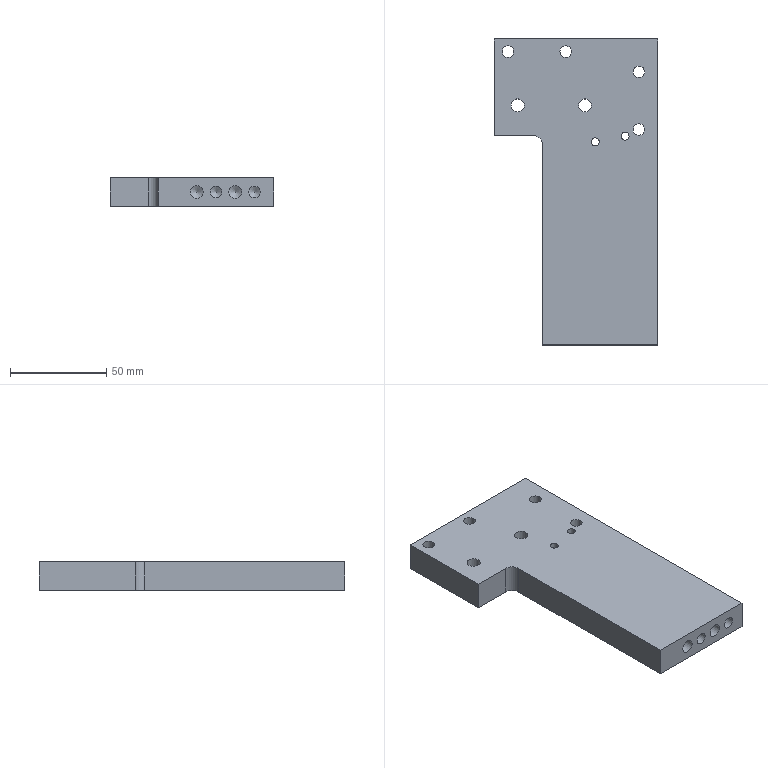Part | NX | features BREP 1 | 1 solid | 33 faces | box 85 x 159 x 15 mm | volume 154336 mm3 | cylinder 17 | plane 8 | cone 8 | commonest cylinder face diameters 6 x8 6.8 x6 4.2 x2 10 x1
STEP:
#1=CARTESIAN_POINT('',(-35.,-79.5,7.5));
#2=VERTEX_POINT('',#1);
#3=CARTESIAN_POINT('',(-35.,24.5,7.5));
#4=VERTEX_POINT('',#3);
#5=CARTESIAN_POINT('',(-35.,79.5,7.5));
#6=DIRECTION('',(0.,1.,0.));
#7=VECTOR('',#6,1000.);
#8=LINE('',#5,#7);
#9=EDGE_CURVE('',#2,#4,#8,.T.);
#10=ORIENTED_EDGE('',*,*,#9,.T.);
#11=CARTESIAN_POINT('',(-35.,24.5,-7.5));
#12=VERTEX_POINT('',#11);
#13=CARTESIAN_POINT('',(-35.,24.5,0.));
#14=DIRECTION('',(0.,0.,-1.));
#15=VECTOR('',#14,1000.);
#16=LINE('',#13,#15);
#17=EDGE_CURVE('',#4,#12,#16,.T.);
#18=ORIENTED_EDGE('',*,*,#17,.T.);
#19=CARTESIAN_POINT('',(-35.,-79.5,-7.5));
#20=VERTEX_POINT('',#19);
#21=CARTESIAN_POINT('',(-35.,79.5,-7.5));
#22=DIRECTION('',(0.,-1.,0.));
#23=VECTOR('',#22,1000.);
#24=LINE('',#21,#23);
#25=EDGE_CURVE('',#12,#20,#24,.T.);
#26=ORIENTED_EDGE('',*,*,#25,.T.);
#27=CARTESIAN_POINT('',(-35.,-79.5,7.5));
#28=DIRECTION('',(0.,0.,1.));
#29=VECTOR('',#28,1000.);
#30=LINE('',#27,#29);
#31=EDGE_CURVE('',#20,#2,#30,.T.);
#32=ORIENTED_EDGE('',*,*,#31,.T.);
#33=EDGE_LOOP('',(#10,#18,#26,#32));
#34=FACE_BOUND('',#33,.T.);
#35=CARTESIAN_POINT('',(-35.,0.,0.));
#36=DIRECTION('',(1.,0.,0.));
#37=DIRECTION('',(0.,0.,1.));
#38=AXIS2_PLACEMENT_3D('',#35,#36,#37);
#39=PLANE('',#38);
#40=ADVANCED_FACE('',(#34),#39,.F.);
#41=CARTESIAN_POINT('',(25.,-79.5,-7.5));
#42=VERTEX_POINT('',#41);
#43=CARTESIAN_POINT('',(25.,79.5,-7.5));
#44=VERTEX_POINT('',#43);
#45=CARTESIAN_POINT('',(25.,-79.5,-7.5));
#46=DIRECTION('',(0.,1.,0.));
#47=VECTOR('',#46,1000.);
#48=LINE('',#45,#47);
#49=EDGE_CURVE('',#42,#44,#48,.T.);
#50=ORIENTED_EDGE('',*,*,#49,.T.);
#51=CARTESIAN_POINT('',(25.,79.5,7.5));
#52=VERTEX_POINT('',#51);
#53=CARTESIAN_POINT('',(25.,79.5,7.5));
#54=DIRECTION('',(0.,0.,-1.));
#55=VECTOR('',#54,1000.);
#56=LINE('',#53,#55);
#57=EDGE_CURVE('',#52,#44,#56,.T.);
#58=ORIENTED_EDGE('',*,*,#57,.F.);
#59=CARTESIAN_POINT('',(25.,-79.5,7.5));
#60=VERTEX_POINT('',#59);
#61=CARTESIAN_POINT('',(25.,-79.5,7.5));
#62=DIRECTION('',(0.,1.,0.));
#63=VECTOR('',#62,1000.);
#64=LINE('',#61,#63);
#65=EDGE_CURVE('',#60,#52,#64,.T.);
#66=ORIENTED_EDGE('',*,*,#65,.F.);
#67=CARTESIAN_POINT('',(25.,-79.5,7.5));
#68=DIRECTION('',(0.,0.,-1.));
#69=VECTOR('',#68,1000.);
#70=LINE('',#67,#69);
#71=EDGE_CURVE('',#60,#42,#70,.T.);
#72=ORIENTED_EDGE('',*,*,#71,.T.);
#73=EDGE_LOOP('',(#50,#58,#66,#72));
#74=FACE_BOUND('',#73,.T.);
#75=CARTESIAN_POINT('',(25.,-79.5,7.5));
#76=DIRECTION('',(-1.,0.,0.));
#77=DIRECTION('',(0.,0.,-1.));
#78=AXIS2_PLACEMENT_3D('',#75,#76,#77);
#79=PLANE('',#78);
#80=ADVANCED_FACE('',(#74),#79,.F.);
#81=CARTESIAN_POINT('',(-5.,79.5,3.));
#82=VERTEX_POINT('',#81);
#83=CARTESIAN_POINT('',(-5.,79.5,0.));
#84=DIRECTION('',(0.,1.,0.));
#85=DIRECTION('',(0.,0.,1.));
#86=AXIS2_PLACEMENT_3D('',#83,#84,#85);
#87=CIRCLE('',#86,3.);
#88=EDGE_CURVE('',#82,#82,#87,.T.);
#89=ORIENTED_EDGE('',*,*,#88,.F.);
#90=EDGE_LOOP('',(#89));
#91=FACE_BOUND('',#90,.T.);
#92=CARTESIAN_POINT('',(15.,79.5,3.));
#93=VERTEX_POINT('',#92);
#94=CARTESIAN_POINT('',(15.,79.5,0.));
#95=DIRECTION('',(0.,1.,0.));
#96=DIRECTION('',(0.,0.,1.));
#97=AXIS2_PLACEMENT_3D('',#94,#95,#96);
#98=CIRCLE('',#97,3.);
#99=EDGE_CURVE('',#93,#93,#98,.T.);
#100=ORIENTED_EDGE('',*,*,#99,.F.);
#101=EDGE_LOOP('',(#100));
#102=FACE_BOUND('',#101,.T.);
#103=CARTESIAN_POINT('',(-15.,79.5,3.4));
#104=VERTEX_POINT('',#103);
#105=CARTESIAN_POINT('',(-15.,79.5,0.));
#106=DIRECTION('',(0.,1.,0.));
#107=DIRECTION('',(0.,0.,1.));
#108=AXIS2_PLACEMENT_3D('',#105,#106,#107);
#109=CIRCLE('',#108,3.4);
#110=EDGE_CURVE('',#104,#104,#109,.T.);
#111=ORIENTED_EDGE('',*,*,#110,.F.);
#112=EDGE_LOOP('',(#111));
#113=FACE_BOUND('',#112,.T.);
#114=CARTESIAN_POINT('',(5.,79.5,3.4));
#115=VERTEX_POINT('',#114);
#116=CARTESIAN_POINT('',(5.,79.5,0.));
#117=DIRECTION('',(0.,1.,0.));
#118=DIRECTION('',(0.,0.,1.));
#119=AXIS2_PLACEMENT_3D('',#116,#117,#118);
#120=CIRCLE('',#119,3.4);
#121=EDGE_CURVE('',#115,#115,#120,.T.);
#122=ORIENTED_EDGE('',*,*,#121,.F.);
#123=EDGE_LOOP('',(#122));
#124=FACE_BOUND('',#123,.T.);
#125=CARTESIAN_POINT('',(-60.,79.5,-7.5));
#126=VERTEX_POINT('',#125);
#127=CARTESIAN_POINT('',(-25.,79.5,-7.5));
#128=DIRECTION('',(-1.,0.,0.));
#129=VECTOR('',#128,1000.);
#130=LINE('',#127,#129);
#131=EDGE_CURVE('',#44,#126,#130,.T.);
#132=ORIENTED_EDGE('',*,*,#131,.T.);
#133=CARTESIAN_POINT('',(-60.,79.5,7.5));
#134=VERTEX_POINT('',#133);
#135=CARTESIAN_POINT('',(-60.,79.5,-63.402));
#136=DIRECTION('',(0.,0.,1.));
#137=VECTOR('',#136,1000.);
#138=LINE('',#135,#137);
#139=EDGE_CURVE('',#126,#134,#138,.T.);
#140=ORIENTED_EDGE('',*,*,#139,.T.);
#141=CARTESIAN_POINT('',(-25.,79.5,7.5));
#142=DIRECTION('',(-1.,0.,0.));
#143=VECTOR('',#142,1000.);
#144=LINE('',#141,#143);
#145=EDGE_CURVE('',#52,#134,#144,.T.);
#146=ORIENTED_EDGE('',*,*,#145,.F.);
#147=ORIENTED_EDGE('',*,*,#57,.T.);
#148=EDGE_LOOP('',(#132,#140,#146,#147));
#149=FACE_BOUND('',#148,.T.);
#150=CARTESIAN_POINT('',(-25.,79.5,7.5));
#151=DIRECTION('',(0.,-1.,0.));
#152=DIRECTION('',(0.,0.,1.));
#153=AXIS2_PLACEMENT_3D('',#150,#151,#152);
#154=PLANE('',#153);
#155=ADVANCED_FACE('',(#91,#102,#113,#124,#149),#154,.F.);
#156=CARTESIAN_POINT('',(-5.,-79.5,-3.));
#157=VERTEX_POINT('',#156);
#158=CARTESIAN_POINT('',(-5.,-79.5,0.));
#159=DIRECTION('',(0.,-1.,0.));
#160=DIRECTION('',(0.,0.,-1.));
#161=AXIS2_PLACEMENT_3D('',#158,#159,#160);
#162=CIRCLE('',#161,3.);
#163=EDGE_CURVE('',#157,#157,#162,.T.);
#164=ORIENTED_EDGE('',*,*,#163,.F.);
#165=EDGE_LOOP('',(#164));
#166=FACE_BOUND('',#165,.T.);
#167=CARTESIAN_POINT('',(15.,-79.5,-3.));
#168=VERTEX_POINT('',#167);
#169=CARTESIAN_POINT('',(15.,-79.5,0.));
#170=DIRECTION('',(0.,-1.,0.));
#171=DIRECTION('',(0.,0.,-1.));
#172=AXIS2_PLACEMENT_3D('',#169,#170,#171);
#173=CIRCLE('',#172,3.);
#174=EDGE_CURVE('',#168,#168,#173,.T.);
#175=ORIENTED_EDGE('',*,*,#174,.F.);
#176=EDGE_LOOP('',(#175));
#177=FACE_BOUND('',#176,.T.);
#178=CARTESIAN_POINT('',(-15.,-79.5,-3.4));
#179=VERTEX_POINT('',#178);
#180=CARTESIAN_POINT('',(-15.,-79.5,0.));
#181=DIRECTION('',(0.,-1.,0.));
#182=DIRECTION('',(0.,0.,-1.));
#183=AXIS2_PLACEMENT_3D('',#180,#181,#182);
#184=CIRCLE('',#183,3.4);
#185=EDGE_CURVE('',#179,#179,#184,.T.);
#186=ORIENTED_EDGE('',*,*,#185,.F.);
#187=EDGE_LOOP('',(#186));
#188=FACE_BOUND('',#187,.T.);
#189=CARTESIAN_POINT('',(5.,-79.5,-3.4));
#190=VERTEX_POINT('',#189);
#191=CARTESIAN_POINT('',(5.,-79.5,0.));
#192=DIRECTION('',(0.,-1.,0.));
#193=DIRECTION('',(0.,0.,-1.));
#194=AXIS2_PLACEMENT_3D('',#191,#192,#193);
#195=CIRCLE('',#194,3.4);
#196=EDGE_CURVE('',#190,#190,#195,.T.);
#197=ORIENTED_EDGE('',*,*,#196,.F.);
#198=EDGE_LOOP('',(#197));
#199=FACE_BOUND('',#198,.T.);
#200=CARTESIAN_POINT('',(-25.,-79.5,-7.5));
#201=DIRECTION('',(1.,0.,0.));
#202=VECTOR('',#201,1000.);
#203=LINE('',#200,#202);
#204=EDGE_CURVE('',#20,#42,#203,.T.);
#205=ORIENTED_EDGE('',*,*,#204,.T.);
#206=ORIENTED_EDGE('',*,*,#71,.F.);
#207=CARTESIAN_POINT('',(-25.,-79.5,7.5));
#208=DIRECTION('',(1.,0.,0.));
#209=VECTOR('',#208,1000.);
#210=LINE('',#207,#209);
#211=EDGE_CURVE('',#2,#60,#210,.T.);
#212=ORIENTED_EDGE('',*,*,#211,.F.);
#213=ORIENTED_EDGE('',*,*,#31,.F.);
#214=EDGE_LOOP('',(#205,#206,#212,#213));
#215=FACE_BOUND('',#214,.T.);
#216=CARTESIAN_POINT('',(-25.,-79.5,7.5));
#217=DIRECTION('',(0.,1.,0.));
#218=DIRECTION('',(0.,0.,-1.));
#219=AXIS2_PLACEMENT_3D('',#216,#217,#218);
#220=PLANE('',#219);
#221=ADVANCED_FACE('',(#166,#177,#188,#199,#215),#220,.F.);
#222=CARTESIAN_POINT('',(5.9,29.,7.5));
#223=VERTEX_POINT('',#222);
#224=CARTESIAN_POINT('',(8.,29.,7.5));
#225=DIRECTION('',(0.,0.,-1.));
#226=DIRECTION('',(-1.,0.,0.));
#227=AXIS2_PLACEMENT_3D('',#224,#225,#226);
#228=CIRCLE('',#227,2.1);
#229=EDGE_CURVE('',#223,#223,#228,.T.);
#230=ORIENTED_EDGE('',*,*,#229,.T.);
#231=EDGE_LOOP('',(#230));
#232=FACE_BOUND('',#231,.T.);
#233=CARTESIAN_POINT('',(-9.6,26.,7.5));
#234=VERTEX_POINT('',#233);
#235=CARTESIAN_POINT('',(-7.5,26.,7.5));
#236=DIRECTION('',(0.,0.,-1.));
#237=DIRECTION('',(-1.,0.,0.));
#238=AXIS2_PLACEMENT_3D('',#235,#236,#237);
#239=CIRCLE('',#238,2.1);
#240=EDGE_CURVE('',#234,#234,#239,.T.);
#241=ORIENTED_EDGE('',*,*,#240,.T.);
#242=EDGE_LOOP('',(#241));
#243=FACE_BOUND('',#242,.T.);
#244=CARTESIAN_POINT('',(-44.42,44.946,7.5));
#245=VERTEX_POINT('',#244);
#246=CARTESIAN_POINT('',(-47.82,44.946,7.5));
#247=DIRECTION('',(0.,0.,1.));
#248=DIRECTION('',(1.,0.,0.));
#249=AXIS2_PLACEMENT_3D('',#246,#247,#248);
#250=CIRCLE('',#249,3.4);
#251=EDGE_CURVE('',#245,#245,#250,.T.);
#252=ORIENTED_EDGE('',*,*,#251,.F.);
#253=EDGE_LOOP('',(#252));
#254=FACE_BOUND('',#253,.T.);
#255=CARTESIAN_POINT('',(-9.42,44.946,7.5));
#256=VERTEX_POINT('',#255);
#257=CARTESIAN_POINT('',(-12.82,44.946,7.5));
#258=DIRECTION('',(0.,0.,1.));
#259=DIRECTION('',(1.,0.,0.));
#260=AXIS2_PLACEMENT_3D('',#257,#258,#259);
#261=CIRCLE('',#260,3.4);
#262=EDGE_CURVE('',#256,#256,#261,.T.);
#263=ORIENTED_EDGE('',*,*,#262,.F.);
#264=EDGE_LOOP('',(#263));
#265=FACE_BOUND('',#264,.T.);
#266=CARTESIAN_POINT('',(-49.82,72.946,7.5));
#267=VERTEX_POINT('',#266);
#268=CARTESIAN_POINT('',(-52.82,72.946,7.5));
#269=DIRECTION('',(0.,0.,1.));
#270=DIRECTION('',(1.,0.,0.));
#271=AXIS2_PLACEMENT_3D('',#268,#269,#270);
#272=CIRCLE('',#271,3.);
#273=EDGE_CURVE('',#267,#267,#272,.T.);
#274=ORIENTED_EDGE('',*,*,#273,.F.);
#275=EDGE_LOOP('',(#274));
#276=FACE_BOUND('',#275,.T.);
#277=CARTESIAN_POINT('',(-19.82,72.946,7.5));
#278=VERTEX_POINT('',#277);
#279=CARTESIAN_POINT('',(-22.82,72.946,7.5));
#280=DIRECTION('',(0.,0.,1.));
#281=DIRECTION('',(1.,0.,0.));
#282=AXIS2_PLACEMENT_3D('',#279,#280,#281);
#283=CIRCLE('',#282,3.);
#284=EDGE_CURVE('',#278,#278,#283,.T.);
#285=ORIENTED_EDGE('',*,*,#284,.F.);
#286=EDGE_LOOP('',(#285));
#287=FACE_BOUND('',#286,.T.);
#288=CARTESIAN_POINT('',(18.18,62.446,7.5));
#289=VERTEX_POINT('',#288);
#290=CARTESIAN_POINT('',(15.18,62.446,7.5));
#291=DIRECTION('',(0.,0.,1.));
#292=DIRECTION('',(1.,0.,0.));
#293=AXIS2_PLACEMENT_3D('',#290,#291,#292);
#294=CIRCLE('',#293,3.);
#295=EDGE_CURVE('',#289,#289,#294,.T.);
#296=ORIENTED_EDGE('',*,*,#295,.F.);
#297=EDGE_LOOP('',(#296));
#298=FACE_BOUND('',#297,.T.);
#299=CARTESIAN_POINT('',(18.18,32.446,7.5));
#300=VERTEX_POINT('',#299);
#301=CARTESIAN_POINT('',(15.18,32.446,7.5));
#302=DIRECTION('',(0.,0.,1.));
#303=DIRECTION('',(1.,0.,0.));
#304=AXIS2_PLACEMENT_3D('',#301,#302,#303);
#305=CIRCLE('',#304,3.);
#306=EDGE_CURVE('',#300,#300,#305,.T.);
#307=ORIENTED_EDGE('',*,*,#306,.F.);
#308=EDGE_LOOP('',(#307));
#309=FACE_BOUND('',#308,.T.);
#310=ORIENTED_EDGE('',*,*,#65,.T.);
#311=ORIENTED_EDGE('',*,*,#145,.T.);
#312=CARTESIAN_POINT('',(-60.,29.5,7.5));
#313=VERTEX_POINT('',#312);
#314=CARTESIAN_POINT('',(-60.,79.5,7.5));
#315=DIRECTION('',(0.,-1.,0.));
#316=VECTOR('',#315,1000.);
#317=LINE('',#314,#316);
#318=EDGE_CURVE('',#134,#313,#317,.T.);
#319=ORIENTED_EDGE('',*,*,#318,.T.);
#320=CARTESIAN_POINT('',(-40.,29.5,7.5));
#321=VERTEX_POINT('',#320);
#322=CARTESIAN_POINT('',(-35.,29.5,7.5));
#323=DIRECTION('',(1.,0.,0.));
#324=VECTOR('',#323,1000.);
#325=LINE('',#322,#324);
#326=EDGE_CURVE('',#313,#321,#325,.T.);
#327=ORIENTED_EDGE('',*,*,#326,.T.);
#328=CARTESIAN_POINT('',(-40.,24.5,7.5));
#329=DIRECTION('',(0.,0.,-1.));
#330=DIRECTION('',(-1.,0.,0.));
#331=AXIS2_PLACEMENT_3D('',#328,#329,#330);
#332=CIRCLE('',#331,5.);
#333=EDGE_CURVE('',#321,#4,#332,.T.);
#334=ORIENTED_EDGE('',*,*,#333,.T.);
#335=ORIENTED_EDGE('',*,*,#9,.F.);
#336=ORIENTED_EDGE('',*,*,#211,.T.);
#337=EDGE_LOOP('',(#310,#311,#319,#327,#334,#335,#336));
#338=FACE_BOUND('',#337,.T.);
#339=CARTESIAN_POINT('',(0.,0.,7.5));
#340=DIRECTION('',(0.,0.,-1.));
#341=DIRECTION('',(1.,0.,0.));
#342=AXIS2_PLACEMENT_3D('',#339,#340,#341);
#343=PLANE('',#342);
#344=ADVANCED_FACE('',(#232,#243,#254,#265,#276,#287,#298,#309,#338),#343,.F.);
#345=CARTESIAN_POINT('',(5.9,29.,-7.5));
#346=VERTEX_POINT('',#345);
#347=CARTESIAN_POINT('',(8.,29.,-7.5));
#348=DIRECTION('',(0.,0.,-1.));
#349=DIRECTION('',(-1.,0.,0.));
#350=AXIS2_PLACEMENT_3D('',#347,#348,#349);
#351=CIRCLE('',#350,2.1);
#352=EDGE_CURVE('',#346,#346,#351,.T.);
#353=ORIENTED_EDGE('',*,*,#352,.F.);
#354=EDGE_LOOP('',(#353));
#355=FACE_BOUND('',#354,.T.);
#356=CARTESIAN_POINT('',(-9.6,26.,-7.5));
#357=VERTEX_POINT('',#356);
#358=CARTESIAN_POINT('',(-7.5,26.,-7.5));
#359=DIRECTION('',(0.,0.,-1.));
#360=DIRECTION('',(-1.,0.,0.));
#361=AXIS2_PLACEMENT_3D('',#358,#359,#360);
#362=CIRCLE('',#361,2.1);
#363=EDGE_CURVE('',#357,#357,#362,.T.);
#364=ORIENTED_EDGE('',*,*,#363,.F.);
#365=EDGE_LOOP('',(#364));
#366=FACE_BOUND('',#365,.T.);
#367=CARTESIAN_POINT('',(-44.42,44.946,-7.5));
#368=VERTEX_POINT('',#367);
#369=CARTESIAN_POINT('',(-47.82,44.946,-7.5));
#370=DIRECTION('',(0.,0.,1.));
#371=DIRECTION('',(1.,0.,0.));
#372=AXIS2_PLACEMENT_3D('',#369,#370,#371);
#373=CIRCLE('',#372,3.4);
#374=EDGE_CURVE('',#368,#368,#373,.T.);
#375=ORIENTED_EDGE('',*,*,#374,.T.);
#376=EDGE_LOOP('',(#375));
#377=FACE_BOUND('',#376,.T.);
#378=CARTESIAN_POINT('',(-9.42,44.946,-7.5));
#379=VERTEX_POINT('',#378);
#380=CARTESIAN_POINT('',(-12.82,44.946,-7.5));
#381=DIRECTION('',(0.,0.,1.));
#382=DIRECTION('',(1.,0.,0.));
#383=AXIS2_PLACEMENT_3D('',#380,#381,#382);
#384=CIRCLE('',#383,3.4);
#385=EDGE_CURVE('',#379,#379,#384,.T.);
#386=ORIENTED_EDGE('',*,*,#385,.T.);
#387=EDGE_LOOP('',(#386));
#388=FACE_BOUND('',#387,.T.);
#389=CARTESIAN_POINT('',(-49.82,72.946,-7.5));
#390=VERTEX_POINT('',#389);
#391=CARTESIAN_POINT('',(-52.82,72.946,-7.5));
#392=DIRECTION('',(0.,0.,1.));
#393=DIRECTION('',(1.,0.,0.));
#394=AXIS2_PLACEMENT_3D('',#391,#392,#393);
#395=CIRCLE('',#394,3.);
#396=EDGE_CURVE('',#390,#390,#395,.T.);
#397=ORIENTED_EDGE('',*,*,#396,.T.);
#398=EDGE_LOOP('',(#397));
#399=FACE_BOUND('',#398,.T.);
#400=CARTESIAN_POINT('',(-19.82,72.946,-7.5));
#401=VERTEX_POINT('',#400);
#402=CARTESIAN_POINT('',(-22.82,72.946,-7.5));
#403=DIRECTION('',(0.,0.,1.));
#404=DIRECTION('',(1.,0.,0.));
#405=AXIS2_PLACEMENT_3D('',#402,#403,#404);
#406=CIRCLE('',#405,3.);
#407=EDGE_CURVE('',#401,#401,#406,.T.);
#408=ORIENTED_EDGE('',*,*,#407,.T.);
#409=EDGE_LOOP('',(#408));
#410=FACE_BOUND('',#409,.T.);
#411=CARTESIAN_POINT('',(18.18,62.446,-7.5));
#412=VERTEX_POINT('',#411);
#413=CARTESIAN_POINT('',(15.18,62.446,-7.5));
#414=DIRECTION('',(0.,0.,1.));
#415=DIRECTION('',(1.,0.,0.));
#416=AXIS2_PLACEMENT_3D('',#413,#414,#415);
#417=CIRCLE('',#416,3.);
#418=EDGE_CURVE('',#412,#412,#417,.T.);
#419=ORIENTED_EDGE('',*,*,#418,.T.);
#420=EDGE_LOOP('',(#419));
#421=FACE_BOUND('',#420,.T.);
#422=CARTESIAN_POINT('',(18.18,32.446,-7.5));
#423=VERTEX_POINT('',#422);
#424=CARTESIAN_POINT('',(15.18,32.446,-7.5));
#425=DIRECTION('',(0.,0.,1.));
#426=DIRECTION('',(1.,0.,0.));
#427=AXIS2_PLACEMENT_3D('',#424,#425,#426);
#428=CIRCLE('',#427,3.);
#429=EDGE_CURVE('',#423,#423,#428,.T.);
#430=ORIENTED_EDGE('',*,*,#429,.T.);
#431=EDGE_LOOP('',(#430));
#432=FACE_BOUND('',#431,.T.);
#433=ORIENTED_EDGE('',*,*,#49,.F.);
#434=ORIENTED_EDGE('',*,*,#204,.F.);
#435=ORIENTED_EDGE('',*,*,#25,.F.);
#436=CARTESIAN_POINT('',(-40.,29.5,-7.5));
#437=VERTEX_POINT('',#436);
#438=CARTESIAN_POINT('',(-40.,24.5,-7.5));
#439=DIRECTION('',(0.,0.,1.));
#440=DIRECTION('',(-1.,0.,0.));
#441=AXIS2_PLACEMENT_3D('',#438,#439,#440);
#442=CIRCLE('',#441,5.);
#443=EDGE_CURVE('',#12,#437,#442,.T.);
#444=ORIENTED_EDGE('',*,*,#443,.T.);
#445=CARTESIAN_POINT('',(-60.,29.5,-7.5));
#446=VERTEX_POINT('',#445);
#447=CARTESIAN_POINT('',(-35.,29.5,-7.5));
#448=DIRECTION('',(1.,0.,0.));
#449=VECTOR('',#448,1000.);
#450=LINE('',#447,#449);
#451=EDGE_CURVE('',#446,#437,#450,.T.);
#452=ORIENTED_EDGE('',*,*,#451,.F.);
#453=CARTESIAN_POINT('',(-60.,79.5,-7.5));
#454=DIRECTION('',(0.,-1.,0.));
#455=VECTOR('',#454,1000.);
#456=LINE('',#453,#455);
#457=EDGE_CURVE('',#126,#446,#456,.T.);
#458=ORIENTED_EDGE('',*,*,#457,.F.);
#459=ORIENTED_EDGE('',*,*,#131,.F.);
#460=EDGE_LOOP('',(#433,#434,#435,#444,#452,#458,#459));
#461=FACE_BOUND('',#460,.T.);
#462=CARTESIAN_POINT('',(0.,0.,-7.5));
#463=DIRECTION('',(0.,0.,-1.));
#464=DIRECTION('',(1.,0.,0.));
#465=AXIS2_PLACEMENT_3D('',#462,#463,#464);
#466=PLANE('',#465);
#467=ADVANCED_FACE('',(#355,#366,#377,#388,#399,#410,#421,#432,#461),#466,.T.);
#468=CARTESIAN_POINT('',(5.,57.707,0.));
#469=VERTEX_POINT('',#468);
#470=VERTEX_LOOP('',#469);
#471=FACE_BOUND('',#470,.T.);
#472=CARTESIAN_POINT('',(5.,59.75,3.4));
#473=VERTEX_POINT('',#472);
#474=CARTESIAN_POINT('',(5.,59.75,0.));
#475=DIRECTION('',(0.,1.,0.));
#476=DIRECTION('',(0.,0.,1.));
#477=AXIS2_PLACEMENT_3D('',#474,#475,#476);
#478=CIRCLE('',#477,3.4);
#479=EDGE_CURVE('',#473,#473,#478,.T.);
#480=ORIENTED_EDGE('',*,*,#479,.T.);
#481=EDGE_LOOP('',(#480));
#482=FACE_BOUND('',#481,.T.);
#483=CARTESIAN_POINT('',(5.,59.75,0.));
#484=DIRECTION('',(0.,1.,0.));
#485=DIRECTION('',(0.,0.,-1.));
#486=AXIS2_PLACEMENT_3D('',#483,#484,#485);
#487=CONICAL_SURFACE('',#486,3.4,1.03);
#488=ADVANCED_FACE('',(#471,#482),#487,.F.);
#489=ORIENTED_EDGE('',*,*,#479,.F.);
#490=EDGE_LOOP('',(#489));
#491=FACE_BOUND('',#490,.T.);
#492=ORIENTED_EDGE('',*,*,#121,.T.);
#493=EDGE_LOOP('',(#492));
#494=FACE_BOUND('',#493,.T.);
#495=CARTESIAN_POINT('',(5.,79.5,0.));
#496=DIRECTION('',(0.,1.,0.));
#497=DIRECTION('',(0.,0.,-1.));
#498=AXIS2_PLACEMENT_3D('',#495,#496,#497);
#499=CYLINDRICAL_SURFACE('',#498,3.4);
#500=ADVANCED_FACE('',(#491,#494),#499,.F.);
#501=CARTESIAN_POINT('',(-15.,57.707,0.));
#502=VERTEX_POINT('',#501);
#503=VERTEX_LOOP('',#502);
#504=FACE_BOUND('',#503,.T.);
#505=CARTESIAN_POINT('',(-15.,59.75,3.4));
#506=VERTEX_POINT('',#505);
#507=CARTESIAN_POINT('',(-15.,59.75,0.));
#508=DIRECTION('',(0.,1.,0.));
#509=DIRECTION('',(0.,0.,1.));
#510=AXIS2_PLACEMENT_3D('',#507,#508,#509);
#511=CIRCLE('',#510,3.4);
#512=EDGE_CURVE('',#506,#506,#511,.T.);
#513=ORIENTED_EDGE('',*,*,#512,.T.);
#514=EDGE_LOOP('',(#513));
#515=FACE_BOUND('',#514,.T.);
#516=CARTESIAN_POINT('',(-15.,59.75,0.));
#517=DIRECTION('',(0.,1.,0.));
#518=DIRECTION('',(0.,0.,-1.));
#519=AXIS2_PLACEMENT_3D('',#516,#517,#518);
#520=CONICAL_SURFACE('',#519,3.4,1.03);
#521=ADVANCED_FACE('',(#504,#515),#520,.F.);
#522=ORIENTED_EDGE('',*,*,#512,.F.);
#523=EDGE_LOOP('',(#522));
#524=FACE_BOUND('',#523,.T.);
#525=ORIENTED_EDGE('',*,*,#110,.T.);
#526=EDGE_LOOP('',(#525));
#527=FACE_BOUND('',#526,.T.);
#528=CARTESIAN_POINT('',(-15.,79.5,0.));
#529=DIRECTION('',(0.,1.,0.));
#530=DIRECTION('',(0.,0.,-1.));
#531=AXIS2_PLACEMENT_3D('',#528,#529,#530);
#532=CYLINDRICAL_SURFACE('',#531,3.4);
#533=ADVANCED_FACE('',(#524,#527),#532,.F.);
#534=CARTESIAN_POINT('',(15.,65.697,0.));
#535=VERTEX_POINT('',#534);
#536=VERTEX_LOOP('',#535);
#537=FACE_BOUND('',#536,.T.);
#538=CARTESIAN_POINT('',(15.,67.5,3.));
#539=VERTEX_POINT('',#538);
#540=CARTESIAN_POINT('',(15.,67.5,0.));
#541=DIRECTION('',(0.,1.,0.));
#542=DIRECTION('',(0.,0.,1.));
#543=AXIS2_PLACEMENT_3D('',#540,#541,#542);
#544=CIRCLE('',#543,3.);
#545=EDGE_CURVE('',#539,#539,#544,.T.);
#546=ORIENTED_EDGE('',*,*,#545,.T.);
#547=EDGE_LOOP('',(#546));
#548=FACE_BOUND('',#547,.T.);
#549=CARTESIAN_POINT('',(15.,67.5,0.));
#550=DIRECTION('',(0.,1.,0.));
#551=DIRECTION('',(0.,0.,-1.));
#552=AXIS2_PLACEMENT_3D('',#549,#550,#551);
#553=CONICAL_SURFACE('',#552,3.,1.03);
#554=ADVANCED_FACE('',(#537,#548),#553,.F.);
#555=ORIENTED_EDGE('',*,*,#545,.F.);
#556=EDGE_LOOP('',(#555));
#557=FACE_BOUND('',#556,.T.);
#558=ORIENTED_EDGE('',*,*,#99,.T.);
#559=EDGE_LOOP('',(#558));
#560=FACE_BOUND('',#559,.T.);
#561=CARTESIAN_POINT('',(15.,79.5,0.));
#562=DIRECTION('',(0.,1.,0.));
#563=DIRECTION('',(0.,0.,-1.));
#564=AXIS2_PLACEMENT_3D('',#561,#562,#563);
#565=CYLINDRICAL_SURFACE('',#564,3.);
#566=ADVANCED_FACE('',(#557,#560),#565,.F.);
#567=CARTESIAN_POINT('',(-5.,65.697,0.));
#568=VERTEX_POINT('',#567);
#569=VERTEX_LOOP('',#568);
#570=FACE_BOUND('',#569,.T.);
#571=CARTESIAN_POINT('',(-5.,67.5,3.));
#572=VERTEX_POINT('',#571);
#573=CARTESIAN_POINT('',(-5.,67.5,0.));
#574=DIRECTION('',(0.,1.,0.));
#575=DIRECTION('',(0.,0.,1.));
#576=AXIS2_PLACEMENT_3D('',#573,#574,#575);
#577=CIRCLE('',#576,3.);
#578=EDGE_CURVE('',#572,#572,#577,.T.);
#579=ORIENTED_EDGE('',*,*,#578,.T.);
#580=EDGE_LOOP('',(#579));
#581=FACE_BOUND('',#580,.T.);
#582=CARTESIAN_POINT('',(-5.,67.5,0.));
#583=DIRECTION('',(0.,1.,0.));
#584=DIRECTION('',(0.,0.,-1.));
#585=AXIS2_PLACEMENT_3D('',#582,#583,#584);
#586=CONICAL_SURFACE('',#585,3.,1.03);
#587=ADVANCED_FACE('',(#570,#581),#586,.F.);
#588=ORIENTED_EDGE('',*,*,#578,.F.);
#589=EDGE_LOOP('',(#588));
#590=FACE_BOUND('',#589,.T.);
#591=ORIENTED_EDGE('',*,*,#88,.T.);
#592=EDGE_LOOP('',(#591));
#593=FACE_BOUND('',#592,.T.);
#594=CARTESIAN_POINT('',(-5.,79.5,0.));
#595=DIRECTION('',(0.,1.,0.));
#596=DIRECTION('',(0.,0.,-1.));
#597=AXIS2_PLACEMENT_3D('',#594,#595,#596);
#598=CYLINDRICAL_SURFACE('',#597,3.);
#599=ADVANCED_FACE('',(#590,#593),#598,.F.);
#600=CARTESIAN_POINT('',(5.,-57.707,0.));
#601=VERTEX_POINT('',#600);
#602=VERTEX_LOOP('',#601);
#603=FACE_BOUND('',#602,.T.);
#604=CARTESIAN_POINT('',(5.,-59.75,-3.4));
#605=VERTEX_POINT('',#604);
#606=CARTESIAN_POINT('',(5.,-59.75,0.));
#607=DIRECTION('',(0.,-1.,0.));
#608=DIRECTION('',(0.,0.,-1.));
#609=AXIS2_PLACEMENT_3D('',#606,#607,#608);
#610=CIRCLE('',#609,3.4);
#611=EDGE_CURVE('',#605,#605,#610,.T.);
#612=ORIENTED_EDGE('',*,*,#611,.T.);
#613=EDGE_LOOP('',(#612));
#614=FACE_BOUND('',#613,.T.);
#615=CARTESIAN_POINT('',(5.,-59.75,0.));
#616=DIRECTION('',(0.,-1.,0.));
#617=DIRECTION('',(0.,0.,1.));
#618=AXIS2_PLACEMENT_3D('',#615,#616,#617);
#619=CONICAL_SURFACE('',#618,3.4,1.03);
#620=ADVANCED_FACE('',(#603,#614),#619,.F.);
#621=ORIENTED_EDGE('',*,*,#611,.F.);
#622=EDGE_LOOP('',(#621));
#623=FACE_BOUND('',#622,.T.);
#624=ORIENTED_EDGE('',*,*,#196,.T.);
#625=EDGE_LOOP('',(#624));
#626=FACE_BOUND('',#625,.T.);
#627=CARTESIAN_POINT('',(5.,-79.5,0.));
#628=DIRECTION('',(0.,-1.,0.));
#629=DIRECTION('',(0.,0.,1.));
#630=AXIS2_PLACEMENT_3D('',#627,#628,#629);
#631=CYLINDRICAL_SURFACE('',#630,3.4);
#632=ADVANCED_FACE('',(#623,#626),#631,.F.);
#633=CARTESIAN_POINT('',(-15.,-57.707,0.));
#634=VERTEX_POINT('',#633);
#635=VERTEX_LOOP('',#634);
#636=FACE_BOUND('',#635,.T.);
#637=CARTESIAN_POINT('',(-15.,-59.75,-3.4));
#638=VERTEX_POINT('',#637);
#639=CARTESIAN_POINT('',(-15.,-59.75,0.));
#640=DIRECTION('',(0.,-1.,0.));
#641=DIRECTION('',(0.,0.,-1.));
#642=AXIS2_PLACEMENT_3D('',#639,#640,#641);
#643=CIRCLE('',#642,3.4);
#644=EDGE_CURVE('',#638,#638,#643,.T.);
#645=ORIENTED_EDGE('',*,*,#644,.T.);
#646=EDGE_LOOP('',(#645));
#647=FACE_BOUND('',#646,.T.);
#648=CARTESIAN_POINT('',(-15.,-59.75,0.));
#649=DIRECTION('',(0.,-1.,0.));
#650=DIRECTION('',(0.,0.,1.));
#651=AXIS2_PLACEMENT_3D('',#648,#649,#650);
#652=CONICAL_SURFACE('',#651,3.4,1.03);
#653=ADVANCED_FACE('',(#636,#647),#652,.F.);
#654=ORIENTED_EDGE('',*,*,#644,.F.);
#655=EDGE_LOOP('',(#654));
#656=FACE_BOUND('',#655,.T.);
#657=ORIENTED_EDGE('',*,*,#185,.T.);
#658=EDGE_LOOP('',(#657));
#659=FACE_BOUND('',#658,.T.);
#660=CARTESIAN_POINT('',(-15.,-79.5,0.));
#661=DIRECTION('',(0.,-1.,0.));
#662=DIRECTION('',(0.,0.,1.));
#663=AXIS2_PLACEMENT_3D('',#660,#661,#662);
#664=CYLINDRICAL_SURFACE('',#663,3.4);
#665=ADVANCED_FACE('',(#656,#659),#664,.F.);
#666=CARTESIAN_POINT('',(15.,-65.697,0.));
#667=VERTEX_POINT('',#666);
#668=VERTEX_LOOP('',#667);
#669=FACE_BOUND('',#668,.T.);
#670=CARTESIAN_POINT('',(15.,-67.5,-3.));
#671=VERTEX_POINT('',#670);
#672=CARTESIAN_POINT('',(15.,-67.5,0.));
#673=DIRECTION('',(0.,-1.,0.));
#674=DIRECTION('',(0.,0.,-1.));
#675=AXIS2_PLACEMENT_3D('',#672,#673,#674);
#676=CIRCLE('',#675,3.);
#677=EDGE_CURVE('',#671,#671,#676,.T.);
#678=ORIENTED_EDGE('',*,*,#677,.T.);
#679=EDGE_LOOP('',(#678));
#680=FACE_BOUND('',#679,.T.);
#681=CARTESIAN_POINT('',(15.,-67.5,0.));
#682=DIRECTION('',(0.,-1.,0.));
#683=DIRECTION('',(0.,0.,1.));
#684=AXIS2_PLACEMENT_3D('',#681,#682,#683);
#685=CONICAL_SURFACE('',#684,3.,1.03);
#686=ADVANCED_FACE('',(#669,#680),#685,.F.);
#687=ORIENTED_EDGE('',*,*,#677,.F.);
#688=EDGE_LOOP('',(#687));
#689=FACE_BOUND('',#688,.T.);
#690=ORIENTED_EDGE('',*,*,#174,.T.);
#691=EDGE_LOOP('',(#690));
#692=FACE_BOUND('',#691,.T.);
#693=CARTESIAN_POINT('',(15.,-79.5,0.));
#694=DIRECTION('',(0.,-1.,0.));
#695=DIRECTION('',(0.,0.,1.));
#696=AXIS2_PLACEMENT_3D('',#693,#694,#695);
#697=CYLINDRICAL_SURFACE('',#696,3.);
#698=ADVANCED_FACE('',(#689,#692),#697,.F.);
#699=CARTESIAN_POINT('',(-5.,-65.697,0.));
#700=VERTEX_POINT('',#699);
#701=VERTEX_LOOP('',#700);
#702=FACE_BOUND('',#701,.T.);
#703=CARTESIAN_POINT('',(-5.,-67.5,-3.));
#704=VERTEX_POINT('',#703);
#705=CARTESIAN_POINT('',(-5.,-67.5,0.));
#706=DIRECTION('',(0.,-1.,0.));
#707=DIRECTION('',(0.,0.,-1.));
#708=AXIS2_PLACEMENT_3D('',#705,#706,#707);
#709=CIRCLE('',#708,3.);
#710=EDGE_CURVE('',#704,#704,#709,.T.);
#711=ORIENTED_EDGE('',*,*,#710,.T.);
#712=EDGE_LOOP('',(#711));
#713=FACE_BOUND('',#712,.T.);
#714=CARTESIAN_POINT('',(-5.,-67.5,0.));
#715=DIRECTION('',(0.,-1.,0.));
#716=DIRECTION('',(0.,0.,1.));
#717=AXIS2_PLACEMENT_3D('',#714,#715,#716);
#718=CONICAL_SURFACE('',#717,3.,1.03);
#719=ADVANCED_FACE('',(#702,#713),#718,.F.);
#720=ORIENTED_EDGE('',*,*,#710,.F.);
#721=EDGE_LOOP('',(#720));
#722=FACE_BOUND('',#721,.T.);
#723=ORIENTED_EDGE('',*,*,#163,.T.);
#724=EDGE_LOOP('',(#723));
#725=FACE_BOUND('',#724,.T.);
#726=CARTESIAN_POINT('',(-5.,-79.5,0.));
#727=DIRECTION('',(0.,-1.,0.));
#728=DIRECTION('',(0.,0.,1.));
#729=AXIS2_PLACEMENT_3D('',#726,#727,#728);
#730=CYLINDRICAL_SURFACE('',#729,3.);
#731=ADVANCED_FACE('',(#722,#725),#730,.F.);
#732=ORIENTED_EDGE('',*,*,#139,.F.);
#733=ORIENTED_EDGE('',*,*,#457,.T.);
#734=CARTESIAN_POINT('',(-60.,29.5,-63.402));
#735=DIRECTION('',(0.,0.,1.));
#736=VECTOR('',#735,1000.);
#737=LINE('',#734,#736);
#738=EDGE_CURVE('',#446,#313,#737,.T.);
#739=ORIENTED_EDGE('',*,*,#738,.T.);
#740=ORIENTED_EDGE('',*,*,#318,.F.);
#741=EDGE_LOOP('',(#732,#733,#739,#740));
#742=FACE_BOUND('',#741,.T.);
#743=CARTESIAN_POINT('',(-60.,79.5,-63.402));
#744=DIRECTION('',(-1.,0.,0.));
#745=DIRECTION('',(0.,0.,-1.));
#746=AXIS2_PLACEMENT_3D('',#743,#744,#745);
#747=PLANE('',#746);
#748=ADVANCED_FACE('',(#742),#747,.T.);
#749=ORIENTED_EDGE('',*,*,#451,.T.);
#750=CARTESIAN_POINT('',(-40.,29.5,-63.402));
#751=DIRECTION('',(0.,0.,1.));
#752=VECTOR('',#751,1000.);
#753=LINE('',#750,#752);
#754=EDGE_CURVE('',#437,#321,#753,.T.);
#755=ORIENTED_EDGE('',*,*,#754,.T.);
#756=ORIENTED_EDGE('',*,*,#326,.F.);
#757=ORIENTED_EDGE('',*,*,#738,.F.);
#758=EDGE_LOOP('',(#749,#755,#756,#757));
#759=FACE_BOUND('',#758,.T.);
#760=CARTESIAN_POINT('',(-35.,29.5,-63.402));
#761=DIRECTION('',(0.,-1.,0.));
#762=DIRECTION('',(0.,0.,1.));
#763=AXIS2_PLACEMENT_3D('',#760,#761,#762);
#764=PLANE('',#763);
#765=ADVANCED_FACE('',(#759),#764,.T.);
#766=ORIENTED_EDGE('',*,*,#443,.F.);
#767=ORIENTED_EDGE('',*,*,#17,.F.);
#768=ORIENTED_EDGE('',*,*,#333,.F.);
#769=ORIENTED_EDGE('',*,*,#754,.F.);
#770=EDGE_LOOP('',(#766,#767,#768,#769));
#771=FACE_BOUND('',#770,.T.);
#772=CARTESIAN_POINT('',(-40.,24.5,-63.402));
#773=DIRECTION('',(0.,0.,1.));
#774=DIRECTION('',(-1.,0.,0.));
#775=AXIS2_PLACEMENT_3D('',#772,#773,#774);
#776=CYLINDRICAL_SURFACE('',#775,5.);
#777=ADVANCED_FACE('',(#771),#776,.F.);
#778=ORIENTED_EDGE('',*,*,#429,.F.);
#779=EDGE_LOOP('',(#778));
#780=FACE_BOUND('',#779,.T.);
#781=ORIENTED_EDGE('',*,*,#306,.T.);
#782=EDGE_LOOP('',(#781));
#783=FACE_BOUND('',#782,.T.);
#784=CARTESIAN_POINT('',(15.18,32.446,7.5));
#785=DIRECTION('',(0.,0.,1.));
#786=DIRECTION('',(-1.,0.,0.));
#787=AXIS2_PLACEMENT_3D('',#784,#785,#786);
#788=CYLINDRICAL_SURFACE('',#787,3.);
#789=ADVANCED_FACE('',(#780,#783),#788,.F.);
#790=ORIENTED_EDGE('',*,*,#418,.F.);
#791=EDGE_LOOP('',(#790));
#792=FACE_BOUND('',#791,.T.);
#793=ORIENTED_EDGE('',*,*,#295,.T.);
#794=EDGE_LOOP('',(#793));
#795=FACE_BOUND('',#794,.T.);
#796=CARTESIAN_POINT('',(15.18,62.446,7.5));
#797=DIRECTION('',(0.,0.,1.));
#798=DIRECTION('',(-1.,0.,0.));
#799=AXIS2_PLACEMENT_3D('',#796,#797,#798);
#800=CYLINDRICAL_SURFACE('',#799,3.);
#801=ADVANCED_FACE('',(#792,#795),#800,.F.);
#802=ORIENTED_EDGE('',*,*,#407,.F.);
#803=EDGE_LOOP('',(#802));
#804=FACE_BOUND('',#803,.T.);
#805=ORIENTED_EDGE('',*,*,#284,.T.);
#806=EDGE_LOOP('',(#805));
#807=FACE_BOUND('',#806,.T.);
#808=CARTESIAN_POINT('',(-22.82,72.946,7.5));
#809=DIRECTION('',(0.,0.,1.));
#810=DIRECTION('',(-1.,0.,0.));
#811=AXIS2_PLACEMENT_3D('',#808,#809,#810);
#812=CYLINDRICAL_SURFACE('',#811,3.);
#813=ADVANCED_FACE('',(#804,#807),#812,.F.);
#814=ORIENTED_EDGE('',*,*,#396,.F.);
#815=EDGE_LOOP('',(#814));
#816=FACE_BOUND('',#815,.T.);
#817=ORIENTED_EDGE('',*,*,#273,.T.);
#818=EDGE_LOOP('',(#817));
#819=FACE_BOUND('',#818,.T.);
#820=CARTESIAN_POINT('',(-52.82,72.946,7.5));
#821=DIRECTION('',(0.,0.,1.));
#822=DIRECTION('',(-1.,0.,0.));
#823=AXIS2_PLACEMENT_3D('',#820,#821,#822);
#824=CYLINDRICAL_SURFACE('',#823,3.);
#825=ADVANCED_FACE('',(#816,#819),#824,.F.);
#826=ORIENTED_EDGE('',*,*,#385,.F.);
#827=EDGE_LOOP('',(#826));
#828=FACE_BOUND('',#827,.T.);
#829=ORIENTED_EDGE('',*,*,#262,.T.);
#830=EDGE_LOOP('',(#829));
#831=FACE_BOUND('',#830,.T.);
#832=CARTESIAN_POINT('',(-12.82,44.946,7.5));
#833=DIRECTION('',(0.,0.,1.));
#834=DIRECTION('',(-1.,0.,0.));
#835=AXIS2_PLACEMENT_3D('',#832,#833,#834);
#836=CYLINDRICAL_SURFACE('',#835,3.4);
#837=ADVANCED_FACE('',(#828,#831),#836,.F.);
#838=ORIENTED_EDGE('',*,*,#374,.F.);
#839=EDGE_LOOP('',(#838));
#840=FACE_BOUND('',#839,.T.);
#841=ORIENTED_EDGE('',*,*,#251,.T.);
#842=EDGE_LOOP('',(#841));
#843=FACE_BOUND('',#842,.T.);
#844=CARTESIAN_POINT('',(-47.82,44.946,7.5));
#845=DIRECTION('',(0.,0.,1.));
#846=DIRECTION('',(-1.,0.,0.));
#847=AXIS2_PLACEMENT_3D('',#844,#845,#846);
#848=CYLINDRICAL_SURFACE('',#847,3.4);
#849=ADVANCED_FACE('',(#840,#843),#848,.F.);
#850=ORIENTED_EDGE('',*,*,#240,.F.);
#851=EDGE_LOOP('',(#850));
#852=FACE_BOUND('',#851,.T.);
#853=ORIENTED_EDGE('',*,*,#363,.T.);
#854=EDGE_LOOP('',(#853));
#855=FACE_BOUND('',#854,.T.);
#856=CARTESIAN_POINT('',(-7.5,26.,-7.5));
#857=DIRECTION('',(0.,0.,-1.));
#858=DIRECTION('',(1.,0.,0.));
#859=AXIS2_PLACEMENT_3D('',#856,#857,#858);
#860=CYLINDRICAL_SURFACE('',#859,2.1);
#861=ADVANCED_FACE('',(#852,#855),#860,.F.);
#862=ORIENTED_EDGE('',*,*,#229,.F.);
#863=EDGE_LOOP('',(#862));
#864=FACE_BOUND('',#863,.T.);
#865=ORIENTED_EDGE('',*,*,#352,.T.);
#866=EDGE_LOOP('',(#865));
#867=FACE_BOUND('',#866,.T.);
#868=CARTESIAN_POINT('',(8.,29.,-7.5));
#869=DIRECTION('',(0.,0.,-1.));
#870=DIRECTION('',(1.,0.,0.));
#871=AXIS2_PLACEMENT_3D('',#868,#869,#870);
#872=CYLINDRICAL_SURFACE('',#871,2.1);
#873=ADVANCED_FACE('',(#864,#867),#872,.F.);
#874=CLOSED_SHELL('',(#40,#80,#155,#221,#344,#467,#488,#500,#521,#533,#554,#566,#587,#599,#620,#632,#653,#665,#686,#698,#719,#731,#748,#765,#777,#789,#801,#813,#825,#837,#849,#861,#873));
#875=MANIFOLD_SOLID_BREP('',#874);
#876=(LENGTH_UNIT()NAMED_UNIT(*)SI_UNIT(.MILLI.,.METRE.));
#877=UNCERTAINTY_MEASURE_WITH_UNIT(LENGTH_MEASURE(0.00001),#876,'','');
#878=(NAMED_UNIT(*)PLANE_ANGLE_UNIT()SI_UNIT($,.RADIAN.));
#879=(NAMED_UNIT(*)SI_UNIT($,.STERADIAN.)SOLID_ANGLE_UNIT());
#880=(GEOMETRIC_REPRESENTATION_CONTEXT(3)GLOBAL_UNCERTAINTY_ASSIGNED_CONTEXT((#877))GLOBAL_UNIT_ASSIGNED_CONTEXT((#876,#878,#879))REPRESENTATION_CONTEXT('',''));
#881=ADVANCED_BREP_SHAPE_REPRESENTATION('',(#875),#880);